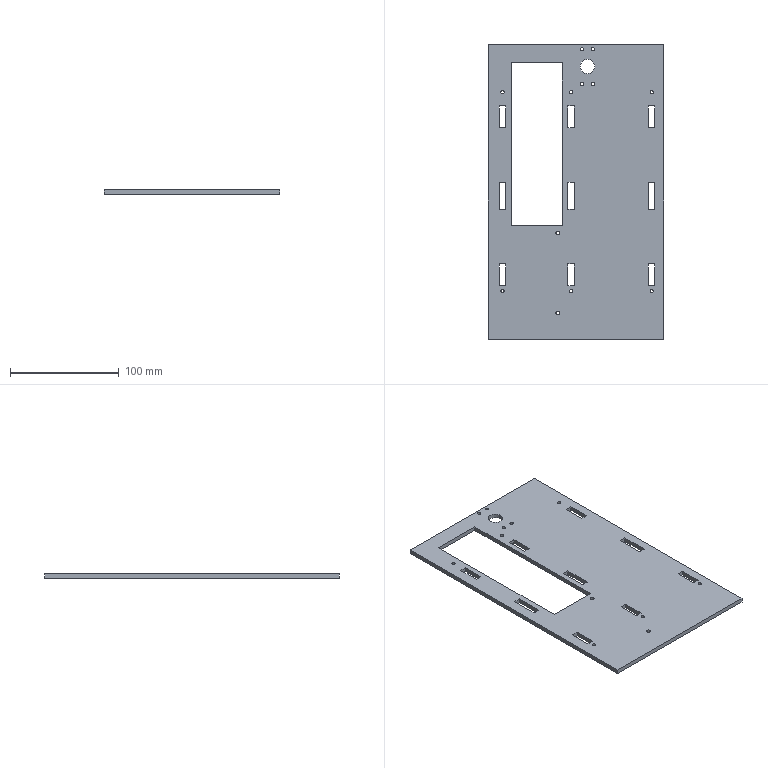Part | SolidWorks | features ICE 34, FlatPattern 1, SMBaseFlange 1, SheetMetal 1 | 1 solid | 74 faces | box 161 x 270 x 4 mm | volume 140085 mm3 | plane 48 | cylinder 26 | commonest cylinder face diameters 3 x20 3.5 x4 13.3 x2